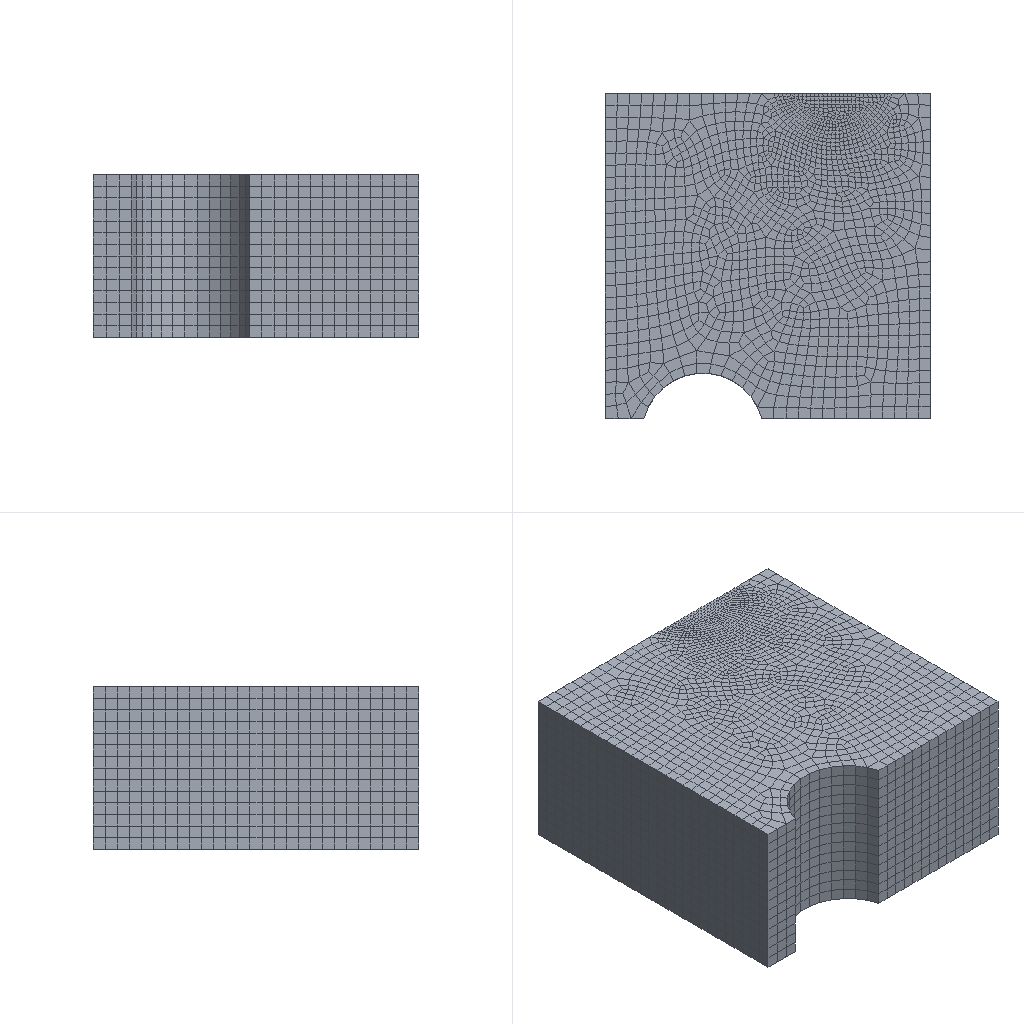Simulation study | abaqus
Set-up summary:
category,name,step,type,value,unit,region
solver,abaqus
solver,version,,,Abaqus/Explicit 2020
units,not stated in the deck,,not stated
analysis,deck,,transient,transient
load_step,Step-1,Step-1,transient,nlgeom=True
contact,interactions,,,general=1 pairs=0 ties=0
load_step,requested,,,1
mesh,nodes,,,27236
mesh,elements,,,24618
element_type,R3D3,,rigid,8
element_type,R3D4,,rigid,1804
element_type,EC3D8R,,solid,22806
load,load commands in deck,,count,1
bc,support commands in deck,,count,12
material,MATERIAL-1,,in results
material,MATERIAL-2,,in results
check,setup vs results,,match,"per instance, exact: element labels, types and connectivity; labels of the nodes the elements use; coordinates of those nodes at SINGLE_PRECISION in 2 of 2 instance(s)"
Abaqus input file, long lists of numbers shortened:
*Heading
** Job name: Job-1 Model name: Model-1
** Generated by: Abaqus/CAE 2020
*Preprint, echo=NO, model=NO, history=NO, contact=NO
**
** PARTS
**
*Part, name=final
*Node
      1,           0.,           0.,         100.
      2,        207.5,           0.,         100.
** (25423 more lines like these left out)
*Element, type=EC3D8R
   1,  1264,  1295,   137,   136,  7765,  7796,  3126,  3127
   2,   950,  1007,  1016,   985,  7451,  7508,  7517,  7486
** (22804 more lines like these left out)
*Nset, nset=Set-1
     1,     2,     3,     4,     5,     6,     7,     8,     9,    10,    11,    12,    13,    14,    15,    16
    19,    20,    25,    26,    27,    28,    29,    30,    31,    32,    33,    34,    35,    36,    37,    38
** (863 more lines like these left out)
*Elset, elset=Set-1
     1,     2,     3,     4,     5,     6,     7,     8,     9,    10,    11,    12,    13,    14,    15,    16
    17,    18,    19,    20,    21,    22,    23,    24,    25,    26,    27,    28,    29,    30,    31,    32
** (711 more lines like these left out)
*Nset, nset=Set-2
     1,     2,     3,     4,     5,     6,     7,     8,     9,    16,    17,    18,    19,    20,    21,    22
    23,    24,    25,    26,    27,    28,    29,    30,    31,    32,    33,    34,    35,    36,    37,    38
** (863 more lines like these left out)
*Elset, elset=Set-2
  9255,  9256,  9257,  9258,  9259,  9260,  9261,  9262,  9263,  9264,  9265,  9266,  9267,  9268,  9269,  9270
  9271,  9272,  9273,  9274,  9275,  9276,  9277,  9278,  9279,  9280,  9281,  9282,  9283,  9284,  9285,  9286
** (711 more lines like these left out)
*Nset, nset=Set-4, generate
     1,  25425,      1
*Elset, elset=Set-4, generate
     1,  22806,      1
*Nset, nset=Set-5, generate
     1,  25425,      1
*Elset, elset=Set-5, generate
     1,  22806,      1
** Section: Section-3
*Eulerian Section, elset=Set-5
Material-1, material-1-1
Material-2, material-2-1
*Surface, type=EULERIAN MATERIAL, name=material-1-1
material-1-1
*Surface, type=EULERIAN MATERIAL, name=material-2-1
material-2-1
*End Part
**
*Part, name=rig
*Node
      1,           8.,  -21.144,           0.
      2,           8.,         105.,           0.
** (1808 more lines like these left out)
*Element, type=R3D4
   1,    1,   27,  114,   28
   2,   27,   26,  115,  114
** (1802 more lines like these left out)
*Element, type=R3D3
1576, 1645, 1643, 1660
1577, 1639, 1629, 1656
** (6 more lines like these left out)
*Node
   1811,           0.,         105., 4.89858741e-16
*Nset, nset=rig-RefPt_, internal
1811,
*Elset, elset=rig, generate
    1,  1812,     1
*End Part
**
**
** ASSEMBLY
**
*Assembly, name=Assembly
**
*Instance, name=rig-1, part=rig
        280.,   -20.797,         100.
*End Instance
**
*Instance, name=final-1, part=final
*End Instance
**
*Nset, nset=Set-1, instance=final-1
     1,     2,     3,     4,     5,     6,     7,     8,     9,    10,    11,    12,    13,    14,    15,    16
    17,    18,    19,    20,    21,    22,    23,    24,    25,    26,    27,    28,    29,    30,    31,    32
** (1304 more lines like these left out)
*Elset, elset=Set-1, instance=final-1, generate
     1,  18508,      1
*Nset, nset=Set-2, instance=final-1
     1,     2,     3,     4,     5,     6,     7,     8,     9,    10,    11,    12,    13,    14,    15,    16
    25,    26,    27,    28,    29,    30,    31,    32,    33,    34,    35,    36,    37,    38,    39,    40
** (695 more lines like these left out)
*Elset, elset=Set-2, instance=final-1, generate
    1,  9254,     1
*Nset, nset=Set-3, instance=final-1
     1,     2,     3,     4,     5,     6,     7,     8,    17,    18,    19,    20,    21,    22,    23,    24
    25,    26,    27,    28,    29,    30,    31,    32,    33,    34,    35,    36,    37,    38,    39,    40
** (695 more lines like these left out)
*Elset, elset=Set-3, instance=final-1, generate
  9255,  18508,      1
*Nset, nset=Set-4, instance=final-1
    1,    2,    3,    4,    5,    6,    7,    8,    9,   10,   11,   12,   13,   14,   15,   16
   17,   18,   19,   20,   21,   22,   23,   24,   25,   26,   27,   28,   29,   30,   31,   32
** (293 more lines like these left out)
*Elset, elset=Set-4, instance=final-1
     1,     4,     7,    16,    22,    25,    56,    57,    74,    76,    77,    78,    89,    90,    91,    93
    94,    95,    96,    97,    98,   110,   112,   113,   114,   115,   121,   139,   206,   335,   363,   367
** (273 more lines like these left out)
*Nset, nset=Set-5, instance=rig-1
 1811,
*Rigid Body, ref node=rig-1.rig-RefPt_, elset=rig-1.rig
*End Assembly
**
** MATERIALS
**
*Material, name=Material-1
*Density
 1.5e-09,
*Elastic
30., 0.35
*Mohr Coulomb
 29.46, 0.1
*Mohr Coulomb Hardening
 0.05458,0.
*Material, name=Material-2
*Density
 1.8e-09,
*Elastic
50., 0.35
*Mohr Coulomb
 32.53, 0.1
*Mohr Coulomb Hardening
 0.1524,0.
**
** INTERACTION PROPERTIES
**
*Surface Interaction, name=IntProp-1
*Friction
 0.2,
*Surface Behavior, pressure-overclosure=HARD
**
** PREDEFINED FIELDS
**
** Name: Predefined Field-1   Type: Material assignment
*Initial Conditions, type=VOLUME FRACTION
Set-2, final-1.material-1-1, 1.
Set-3, final-1.material-2-1, 1.
** ----------------------------------------------------------------
**
** STEP: Step-1
**
*Step, name=Step-1, nlgeom=YES
*Dynamic, Explicit
, 0.04
*Bulk Viscosity
0.06, 1.2
** Mass Scaling: Semi-Automatic
**               Whole Model
*Fixed Mass Scaling, factor=5000.
**
** BOUNDARY CONDITIONS
**
** Name: BC-1 Type: 速度/角速度
*Boundary, type=VELOCITY
Set-4, 1, 1
Set-4, 2, 2
Set-4, 3, 3
Set-4, 4, 4
Set-4, 5, 5
Set-4, 6, 6
** Name: [REDACTED] : Speed/Angular velocity
*Boundary, type=VELOCITY
Set-5, 1, 1
Set-5, 2, 2, -1000.
Set-5, 3, 3
Set-5, 4, 4
Set-5, 5, 5
Set-5, 6, 6
**
** INTERACTIONS
**
** Interaction: Int-1
*Contact, op=NEW
*Contact Inclusions, ALL EXTERIOR
*Contact Property Assignment
 ,  , IntProp-1
**
** OUTPUT REQUESTS
**
*Restart, write, number interval=1, time marks=NO
**
** FIELD OUTPUT: F-Output-1
**
*Output, field, number interval=50
*Node Output
A, COORD, RF, RM, RT, U, V
*Element Output, directions=YES
DENSITY, DENSITYVAVG, E, ESDV, ESOL, EVF, EVOL, FV, IVOL, LE, MISES, MISESMAX, MISESONLY, PE, PEEQ, PEEQMAX
PEEQT, PEEQVAVG, PEVAVG, PRESSONLY, S, SDV, SEQUT, STATUS, STH, SVAVG, SVOL, YIELDPOT
*Contact Output
CDISP, CSTRESS
**
** HISTORY OUTPUT: H-Output-1
**
*Output, history, time interval=2e-06
*Node Output, nset=Set-5
RF1, RF2, RF3
*End Step
Results summary:
result,step,Step-1,completed,increments=3388 time=0.04/0.04
result,analysis,,,transient
result,last_loadstep,,,1
result,analysis steps,,count,1
result,primary field,,,U
result,reaction total,,FX,117.478,model units
result,reaction total,,FY,246.409,model units
result,reaction total,,FZ,-161.612,model units